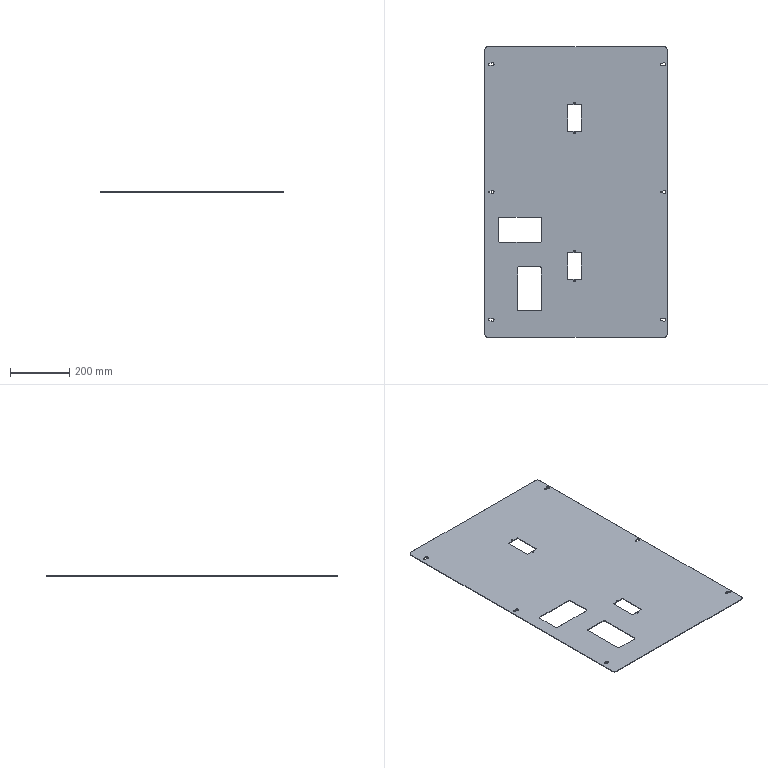Part | SolidWorks | features ICE 6, Fillet 2, Extrusion 1, LPattern 1 | 1 solid | 72 faces | box 615 x 983 x 2 mm | volume 1141777 mm3 | cylinder 38 | plane 34 | commonest cylinder face diameters 6.6 x12 4.5 x8 10 x8 11 x6 20 x4